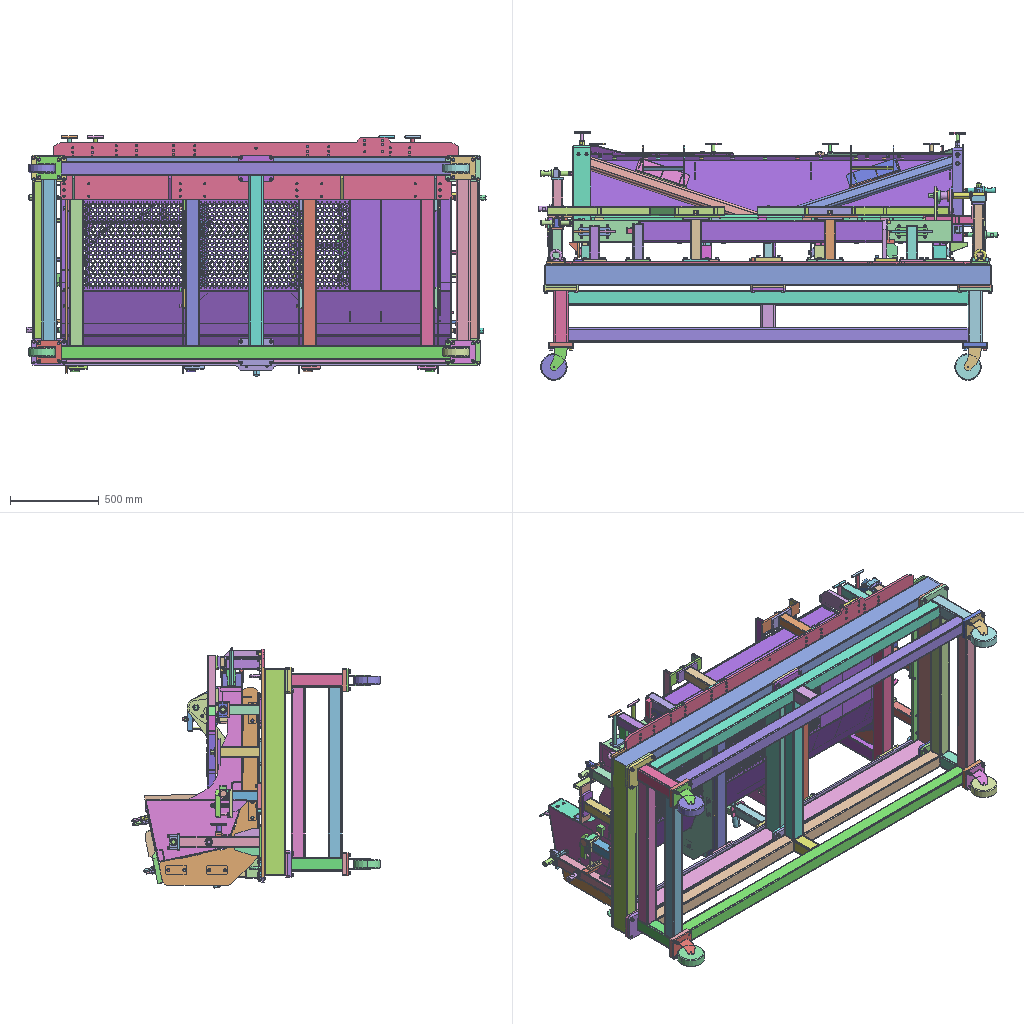Assembly | STEP file | 2 different items | 2 placed | box 2599 x 1406 x 1357 mm
Parts list (item | name | quantity | parent item):
1 | COMPOUND | x1 | in dispositivo de montagem
2 | COMPOUND | x1 | in dispositivo de montagem
Placements (level | parent | child | x y z in mm | rotation matrix by rows):
1 | dispositivo de montagem | COMPOUND | 0.0 0.0 0.0 | 1 0 0 0 1 0 0 0 1
1 | dispositivo de montagem | COMPOUND | 0.0 0.0 0.0 | 1 0 0 0 1 0 0 0 1